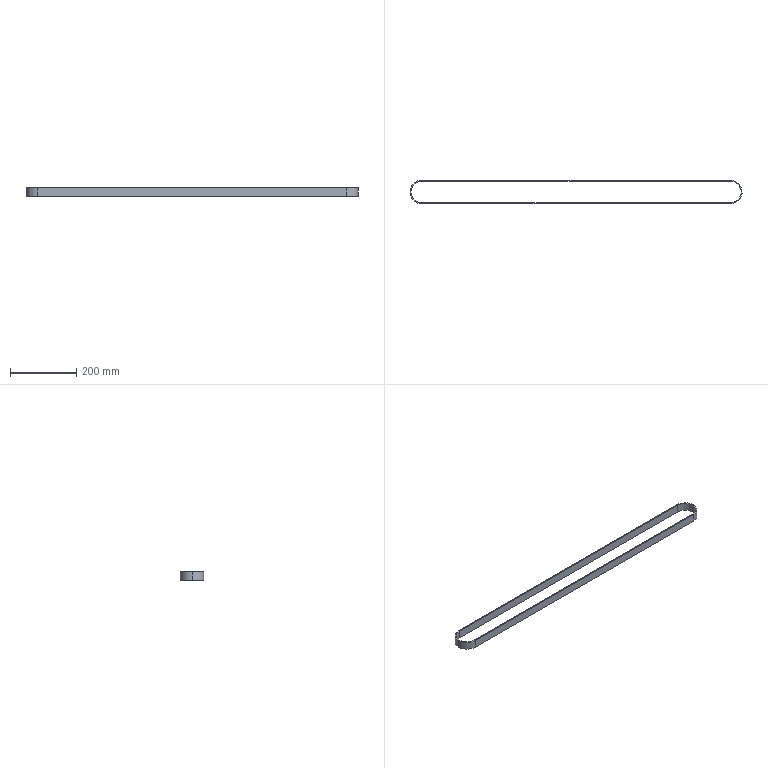Part | STEP file | Timing belt | 1 solid | 12 faces | box 1001 x 71 x 25 mm | volume 155522 mm3 | cylinder 6 | plane 6 | commonest cylinder face diameters 65 x3 71 x3
STEP:
#1=CARTESIAN_POINT('',(-34.001,0.7196,25.));
#2=VERTEX_POINT('',#1);
#3=CARTESIAN_POINT('',(1.594,-34.78,25.));
#4=VERTEX_POINT('',#3);
#5=CARTESIAN_POINT('',(1.499,0.7196,25.));
#6=DIRECTION('',(0.,0.,1.));
#7=DIRECTION('',(-1.,0.,0.));
#8=AXIS2_PLACEMENT_3D('',#5,#6,#7);
#9=CIRCLE('',#8,35.5);
#10=EDGE_CURVE('',#2,#4,#9,.T.);
#11=ORIENTED_EDGE('',*,*,#10,.F.);
#12=CARTESIAN_POINT('',(-34.001,0.7196,0.));
#13=VERTEX_POINT('',#12);
#14=CARTESIAN_POINT('',(-34.001,0.7196,25.));
#15=DIRECTION('',(0.,0.,-1.));
#16=VECTOR('',#15,1000.);
#17=LINE('',#14,#16);
#18=EDGE_CURVE('',#2,#13,#17,.T.);
#19=ORIENTED_EDGE('',*,*,#18,.T.);
#20=CARTESIAN_POINT('',(1.594,-34.78,0.));
#21=VERTEX_POINT('',#20);
#22=CARTESIAN_POINT('',(1.499,0.7196,0.));
#23=DIRECTION('',(0.,0.,1.));
#24=DIRECTION('',(-1.,0.,0.));
#25=AXIS2_PLACEMENT_3D('',#22,#23,#24);
#26=CIRCLE('',#25,35.5);
#27=EDGE_CURVE('',#13,#21,#26,.T.);
#28=ORIENTED_EDGE('',*,*,#27,.T.);
#29=CARTESIAN_POINT('',(1.594,-34.78,25.));
#30=DIRECTION('',(0.,0.,1.));
#31=VECTOR('',#30,1000.);
#32=LINE('',#29,#31);
#33=EDGE_CURVE('',#21,#4,#32,.T.);
#34=ORIENTED_EDGE('',*,*,#33,.T.);
#35=EDGE_LOOP('',(#11,#19,#28,#34));
#36=FACE_OUTER_BOUND('',#35,.T.);
#37=CARTESIAN_POINT('',(1.499,0.7196,25.));
#38=DIRECTION('',(0.,0.,-1.));
#39=DIRECTION('',(-1.,0.,0.));
#40=AXIS2_PLACEMENT_3D('',#37,#38,#39);
#41=CYLINDRICAL_SURFACE('',#40,35.5);
#42=ADVANCED_FACE('',(#36),#41,.T.);
#43=CARTESIAN_POINT('',(-31.001,0.7196,25.));
#44=VERTEX_POINT('',#43);
#45=CARTESIAN_POINT('',(1.411,33.219,25.));
#46=VERTEX_POINT('',#45);
#47=CARTESIAN_POINT('',(1.499,0.7196,25.));
#48=DIRECTION('',(0.,0.,-1.));
#49=DIRECTION('',(-1.,0.,0.));
#50=AXIS2_PLACEMENT_3D('',#47,#48,#49);
#51=CIRCLE('',#50,32.5);
#52=EDGE_CURVE('',#44,#46,#51,.T.);
#53=ORIENTED_EDGE('',*,*,#52,.F.);
#54=CARTESIAN_POINT('',(-31.001,0.7196,0.));
#55=VERTEX_POINT('',#54);
#56=CARTESIAN_POINT('',(-31.001,0.7196,25.));
#57=DIRECTION('',(0.,0.,-1.));
#58=VECTOR('',#57,1000.);
#59=LINE('',#56,#58);
#60=EDGE_CURVE('',#44,#55,#59,.T.);
#61=ORIENTED_EDGE('',*,*,#60,.T.);
#62=CARTESIAN_POINT('',(1.411,33.219,0.));
#63=VERTEX_POINT('',#62);
#64=CARTESIAN_POINT('',(1.499,0.7196,0.));
#65=DIRECTION('',(0.,0.,-1.));
#66=DIRECTION('',(-1.,0.,0.));
#67=AXIS2_PLACEMENT_3D('',#64,#65,#66);
#68=CIRCLE('',#67,32.5);
#69=EDGE_CURVE('',#55,#63,#68,.T.);
#70=ORIENTED_EDGE('',*,*,#69,.T.);
#71=CARTESIAN_POINT('',(1.411,33.219,25.));
#72=DIRECTION('',(0.,0.,-1.));
#73=VECTOR('',#72,1000.);
#74=LINE('',#71,#73);
#75=EDGE_CURVE('',#46,#63,#74,.T.);
#76=ORIENTED_EDGE('',*,*,#75,.F.);
#77=EDGE_LOOP('',(#53,#61,#70,#76));
#78=FACE_OUTER_BOUND('',#77,.T.);
#79=CARTESIAN_POINT('',(1.499,0.7196,25.));
#80=DIRECTION('',(0.,0.,-1.));
#81=DIRECTION('',(-1.,0.,0.));
#82=AXIS2_PLACEMENT_3D('',#79,#80,#81);
#83=CYLINDRICAL_SURFACE('',#82,32.5);
#84=ADVANCED_FACE('',(#78),#83,.F.);
#85=CARTESIAN_POINT('',(931.594,-34.78,25.));
#86=VERTEX_POINT('',#85);
#87=CARTESIAN_POINT('',(931.594,-34.78,0.));
#88=VERTEX_POINT('',#87);
#89=CARTESIAN_POINT('',(931.594,-34.78,25.));
#90=DIRECTION('',(0.,0.,-1.));
#91=VECTOR('',#90,1000.);
#92=LINE('',#89,#91);
#93=EDGE_CURVE('',#86,#88,#92,.T.);
#94=ORIENTED_EDGE('',*,*,#93,.F.);
#95=CARTESIAN_POINT('',(931.594,-34.78,25.));
#96=DIRECTION('',(1.,0.,0.));
#97=VECTOR('',#96,1000.);
#98=LINE('',#95,#97);
#99=EDGE_CURVE('',#4,#86,#98,.T.);
#100=ORIENTED_EDGE('',*,*,#99,.F.);
#101=ORIENTED_EDGE('',*,*,#33,.F.);
#102=CARTESIAN_POINT('',(931.594,-34.78,0.));
#103=DIRECTION('',(-1.,0.,0.));
#104=VECTOR('',#103,1000.);
#105=LINE('',#102,#104);
#106=EDGE_CURVE('',#88,#21,#105,.T.);
#107=ORIENTED_EDGE('',*,*,#106,.F.);
#108=EDGE_LOOP('',(#94,#100,#101,#107));
#109=FACE_OUTER_BOUND('',#108,.T.);
#110=CARTESIAN_POINT('',(931.594,-34.78,25.));
#111=DIRECTION('',(0.,1.,0.));
#112=DIRECTION('',(-1.,0.,0.));
#113=AXIS2_PLACEMENT_3D('',#110,#111,#112);
#114=PLANE('',#113);
#115=ADVANCED_FACE('',(#109),#114,.F.);
#116=CARTESIAN_POINT('',(1.586,-31.78,0.));
#117=VERTEX_POINT('',#116);
#118=CARTESIAN_POINT('',(1.499,0.7196,0.));
#119=DIRECTION('',(0.,0.,-1.));
#120=DIRECTION('',(-1.,0.,0.));
#121=AXIS2_PLACEMENT_3D('',#118,#119,#120);
#122=CIRCLE('',#121,32.5);
#123=EDGE_CURVE('',#117,#55,#122,.T.);
#124=ORIENTED_EDGE('',*,*,#123,.F.);
#125=CARTESIAN_POINT('',(931.586,-31.78,0.));
#126=VERTEX_POINT('',#125);
#127=CARTESIAN_POINT('',(1.499,-31.78,0.));
#128=DIRECTION('',(-1.,0.,0.));
#129=VECTOR('',#128,1000.);
#130=LINE('',#127,#129);
#131=EDGE_CURVE('',#126,#117,#130,.T.);
#132=ORIENTED_EDGE('',*,*,#131,.F.);
#133=CARTESIAN_POINT('',(931.411,33.219,0.));
#134=VERTEX_POINT('',#133);
#135=CARTESIAN_POINT('',(931.499,0.7196,0.));
#136=DIRECTION('',(0.,0.,-1.));
#137=DIRECTION('',(-1.,0.,0.));
#138=AXIS2_PLACEMENT_3D('',#135,#136,#137);
#139=CIRCLE('',#138,32.5);
#140=EDGE_CURVE('',#134,#126,#139,.T.);
#141=ORIENTED_EDGE('',*,*,#140,.F.);
#142=CARTESIAN_POINT('',(1.499,33.219,0.));
#143=DIRECTION('',(1.,0.,0.));
#144=VECTOR('',#143,1000.);
#145=LINE('',#142,#144);
#146=EDGE_CURVE('',#63,#134,#145,.T.);
#147=ORIENTED_EDGE('',*,*,#146,.F.);
#148=ORIENTED_EDGE('',*,*,#69,.F.);
#149=EDGE_LOOP('',(#124,#132,#141,#147,#148));
#150=FACE_BOUND('',#149,.T.);
#151=CARTESIAN_POINT('',(931.403,36.219,0.));
#152=VERTEX_POINT('',#151);
#153=CARTESIAN_POINT('',(1.403,36.219,0.));
#154=VERTEX_POINT('',#153);
#155=CARTESIAN_POINT('',(1.499,36.219,0.));
#156=DIRECTION('',(-1.,0.,0.));
#157=VECTOR('',#156,1000.);
#158=LINE('',#155,#157);
#159=EDGE_CURVE('',#152,#154,#158,.T.);
#160=ORIENTED_EDGE('',*,*,#159,.F.);
#161=CARTESIAN_POINT('',(931.499,0.7196,0.));
#162=DIRECTION('',(0.,0.,1.));
#163=DIRECTION('',(-1.,0.,0.));
#164=AXIS2_PLACEMENT_3D('',#161,#162,#163);
#165=CIRCLE('',#164,35.5);
#166=EDGE_CURVE('',#88,#152,#165,.T.);
#167=ORIENTED_EDGE('',*,*,#166,.F.);
#168=ORIENTED_EDGE('',*,*,#106,.T.);
#169=ORIENTED_EDGE('',*,*,#27,.F.);
#170=CARTESIAN_POINT('',(1.499,0.7196,0.));
#171=DIRECTION('',(0.,0.,1.));
#172=DIRECTION('',(-1.,0.,0.));
#173=AXIS2_PLACEMENT_3D('',#170,#171,#172);
#174=CIRCLE('',#173,35.5);
#175=EDGE_CURVE('',#154,#13,#174,.T.);
#176=ORIENTED_EDGE('',*,*,#175,.F.);
#177=EDGE_LOOP('',(#160,#167,#168,#169,#176));
#178=FACE_OUTER_BOUND('',#177,.T.);
#179=CARTESIAN_POINT('',(1.499,0.7196,0.));
#180=DIRECTION('',(0.,0.,1.));
#181=DIRECTION('',(1.,0.,0.));
#182=AXIS2_PLACEMENT_3D('',#179,#180,#181);
#183=PLANE('',#182);
#184=ADVANCED_FACE('',(#150,#178),#183,.F.);
#185=CARTESIAN_POINT('',(931.403,36.219,25.));
#186=VERTEX_POINT('',#185);
#187=CARTESIAN_POINT('',(931.499,0.7196,25.));
#188=DIRECTION('',(0.,0.,-1.));
#189=DIRECTION('',(-1.,0.,0.));
#190=AXIS2_PLACEMENT_3D('',#187,#188,#189);
#191=CIRCLE('',#190,35.5);
#192=EDGE_CURVE('',#186,#86,#191,.T.);
#193=ORIENTED_EDGE('',*,*,#192,.T.);
#194=ORIENTED_EDGE('',*,*,#93,.T.);
#195=ORIENTED_EDGE('',*,*,#166,.T.);
#196=CARTESIAN_POINT('',(931.403,36.219,25.));
#197=DIRECTION('',(0.,0.,1.));
#198=VECTOR('',#197,1000.);
#199=LINE('',#196,#198);
#200=EDGE_CURVE('',#152,#186,#199,.T.);
#201=ORIENTED_EDGE('',*,*,#200,.T.);
#202=EDGE_LOOP('',(#193,#194,#195,#201));
#203=FACE_OUTER_BOUND('',#202,.T.);
#204=CARTESIAN_POINT('',(931.499,0.7196,25.));
#205=DIRECTION('',(0.,0.,-1.));
#206=DIRECTION('',(-1.,0.,0.));
#207=AXIS2_PLACEMENT_3D('',#204,#205,#206);
#208=CYLINDRICAL_SURFACE('',#207,35.5);
#209=ADVANCED_FACE('',(#203),#208,.T.);
#210=CARTESIAN_POINT('',(931.411,33.219,25.));
#211=VERTEX_POINT('',#210);
#212=CARTESIAN_POINT('',(1.499,33.219,25.));
#213=DIRECTION('',(1.,0.,0.));
#214=VECTOR('',#213,1000.);
#215=LINE('',#212,#214);
#216=EDGE_CURVE('',#46,#211,#215,.T.);
#217=ORIENTED_EDGE('',*,*,#216,.T.);
#218=CARTESIAN_POINT('',(931.586,-31.78,25.));
#219=VERTEX_POINT('',#218);
#220=CARTESIAN_POINT('',(931.499,0.7196,25.));
#221=DIRECTION('',(0.,0.,-1.));
#222=DIRECTION('',(-1.,0.,0.));
#223=AXIS2_PLACEMENT_3D('',#220,#221,#222);
#224=CIRCLE('',#223,32.5);
#225=EDGE_CURVE('',#211,#219,#224,.T.);
#226=ORIENTED_EDGE('',*,*,#225,.T.);
#227=CARTESIAN_POINT('',(1.586,-31.78,25.));
#228=VERTEX_POINT('',#227);
#229=CARTESIAN_POINT('',(1.499,-31.78,25.));
#230=DIRECTION('',(-1.,0.,0.));
#231=VECTOR('',#230,1000.);
#232=LINE('',#229,#231);
#233=EDGE_CURVE('',#219,#228,#232,.T.);
#234=ORIENTED_EDGE('',*,*,#233,.T.);
#235=CARTESIAN_POINT('',(1.499,0.7196,25.));
#236=DIRECTION('',(0.,0.,-1.));
#237=DIRECTION('',(-1.,0.,0.));
#238=AXIS2_PLACEMENT_3D('',#235,#236,#237);
#239=CIRCLE('',#238,32.5);
#240=EDGE_CURVE('',#228,#44,#239,.T.);
#241=ORIENTED_EDGE('',*,*,#240,.T.);
#242=ORIENTED_EDGE('',*,*,#52,.T.);
#243=EDGE_LOOP('',(#217,#226,#234,#241,#242));
#244=FACE_BOUND('',#243,.T.);
#245=ORIENTED_EDGE('',*,*,#192,.F.);
#246=CARTESIAN_POINT('',(1.403,36.219,25.));
#247=VERTEX_POINT('',#246);
#248=CARTESIAN_POINT('',(1.499,36.219,25.));
#249=DIRECTION('',(-1.,0.,0.));
#250=VECTOR('',#249,1000.);
#251=LINE('',#248,#250);
#252=EDGE_CURVE('',#186,#247,#251,.T.);
#253=ORIENTED_EDGE('',*,*,#252,.T.);
#254=CARTESIAN_POINT('',(1.499,0.7196,25.));
#255=DIRECTION('',(0.,0.,1.));
#256=DIRECTION('',(-1.,0.,0.));
#257=AXIS2_PLACEMENT_3D('',#254,#255,#256);
#258=CIRCLE('',#257,35.5);
#259=EDGE_CURVE('',#247,#2,#258,.T.);
#260=ORIENTED_EDGE('',*,*,#259,.T.);
#261=ORIENTED_EDGE('',*,*,#10,.T.);
#262=ORIENTED_EDGE('',*,*,#99,.T.);
#263=EDGE_LOOP('',(#245,#253,#260,#261,#262));
#264=FACE_OUTER_BOUND('',#263,.T.);
#265=CARTESIAN_POINT('',(1.499,0.7196,25.));
#266=DIRECTION('',(0.,0.,1.));
#267=DIRECTION('',(1.,0.,0.));
#268=AXIS2_PLACEMENT_3D('',#265,#266,#267);
#269=PLANE('',#268);
#270=ADVANCED_FACE('',(#244,#264),#269,.T.);
#271=ORIENTED_EDGE('',*,*,#18,.F.);
#272=ORIENTED_EDGE('',*,*,#259,.F.);
#273=CARTESIAN_POINT('',(1.403,36.219,25.));
#274=DIRECTION('',(0.,0.,-1.));
#275=VECTOR('',#274,1000.);
#276=LINE('',#273,#275);
#277=EDGE_CURVE('',#247,#154,#276,.T.);
#278=ORIENTED_EDGE('',*,*,#277,.T.);
#279=ORIENTED_EDGE('',*,*,#175,.T.);
#280=EDGE_LOOP('',(#271,#272,#278,#279));
#281=FACE_OUTER_BOUND('',#280,.T.);
#282=CARTESIAN_POINT('',(1.499,0.7196,25.));
#283=DIRECTION('',(0.,0.,-1.));
#284=DIRECTION('',(-1.,0.,0.));
#285=AXIS2_PLACEMENT_3D('',#282,#283,#284);
#286=CYLINDRICAL_SURFACE('',#285,35.5);
#287=ADVANCED_FACE('',(#281),#286,.T.);
#288=ORIENTED_EDGE('',*,*,#60,.F.);
#289=ORIENTED_EDGE('',*,*,#240,.F.);
#290=CARTESIAN_POINT('',(1.586,-31.78,25.));
#291=DIRECTION('',(0.,0.,1.));
#292=VECTOR('',#291,1000.);
#293=LINE('',#290,#292);
#294=EDGE_CURVE('',#117,#228,#293,.T.);
#295=ORIENTED_EDGE('',*,*,#294,.F.);
#296=ORIENTED_EDGE('',*,*,#123,.T.);
#297=EDGE_LOOP('',(#288,#289,#295,#296));
#298=FACE_OUTER_BOUND('',#297,.T.);
#299=CARTESIAN_POINT('',(1.499,0.7196,25.));
#300=DIRECTION('',(0.,0.,-1.));
#301=DIRECTION('',(-1.,0.,0.));
#302=AXIS2_PLACEMENT_3D('',#299,#300,#301);
#303=CYLINDRICAL_SURFACE('',#302,32.5);
#304=ADVANCED_FACE('',(#298),#303,.F.);
#305=ORIENTED_EDGE('',*,*,#233,.F.);
#306=CARTESIAN_POINT('',(931.586,-31.78,25.));
#307=DIRECTION('',(0.,0.,-1.));
#308=VECTOR('',#307,1000.);
#309=LINE('',#306,#308);
#310=EDGE_CURVE('',#219,#126,#309,.T.);
#311=ORIENTED_EDGE('',*,*,#310,.T.);
#312=ORIENTED_EDGE('',*,*,#131,.T.);
#313=ORIENTED_EDGE('',*,*,#294,.T.);
#314=EDGE_LOOP('',(#305,#311,#312,#313));
#315=FACE_OUTER_BOUND('',#314,.T.);
#316=CARTESIAN_POINT('',(1.586,-31.78,25.));
#317=DIRECTION('',(0.,1.,0.));
#318=DIRECTION('',(-1.,0.,0.));
#319=AXIS2_PLACEMENT_3D('',#316,#317,#318);
#320=PLANE('',#319);
#321=ADVANCED_FACE('',(#315),#320,.T.);
#322=ORIENTED_EDGE('',*,*,#310,.F.);
#323=ORIENTED_EDGE('',*,*,#225,.F.);
#324=CARTESIAN_POINT('',(931.411,33.219,25.));
#325=DIRECTION('',(0.,0.,1.));
#326=VECTOR('',#325,1000.);
#327=LINE('',#324,#326);
#328=EDGE_CURVE('',#134,#211,#327,.T.);
#329=ORIENTED_EDGE('',*,*,#328,.F.);
#330=ORIENTED_EDGE('',*,*,#140,.T.);
#331=EDGE_LOOP('',(#322,#323,#329,#330));
#332=FACE_OUTER_BOUND('',#331,.T.);
#333=CARTESIAN_POINT('',(931.499,0.7196,25.));
#334=DIRECTION('',(0.,0.,-1.));
#335=DIRECTION('',(-1.,0.,0.));
#336=AXIS2_PLACEMENT_3D('',#333,#334,#335);
#337=CYLINDRICAL_SURFACE('',#336,32.5);
#338=ADVANCED_FACE('',(#332),#337,.F.);
#339=ORIENTED_EDGE('',*,*,#216,.F.);
#340=ORIENTED_EDGE('',*,*,#75,.T.);
#341=ORIENTED_EDGE('',*,*,#146,.T.);
#342=ORIENTED_EDGE('',*,*,#328,.T.);
#343=EDGE_LOOP('',(#339,#340,#341,#342));
#344=FACE_OUTER_BOUND('',#343,.T.);
#345=CARTESIAN_POINT('',(1.411,33.219,25.));
#346=DIRECTION('',(0.,-1.,0.));
#347=DIRECTION('',(1.,0.,0.));
#348=AXIS2_PLACEMENT_3D('',#345,#346,#347);
#349=PLANE('',#348);
#350=ADVANCED_FACE('',(#344),#349,.T.);
#351=ORIENTED_EDGE('',*,*,#277,.F.);
#352=ORIENTED_EDGE('',*,*,#252,.F.);
#353=ORIENTED_EDGE('',*,*,#200,.F.);
#354=ORIENTED_EDGE('',*,*,#159,.T.);
#355=EDGE_LOOP('',(#351,#352,#353,#354));
#356=FACE_OUTER_BOUND('',#355,.T.);
#357=CARTESIAN_POINT('',(1.403,36.219,25.));
#358=DIRECTION('',(0.,-1.,0.));
#359=DIRECTION('',(1.,0.,0.));
#360=AXIS2_PLACEMENT_3D('',#357,#358,#359);
#361=PLANE('',#360);
#362=ADVANCED_FACE('',(#356),#361,.F.);
#363=CLOSED_SHELL('',(#42,#84,#115,#184,#209,#270,#287,#304,#321,#338,#350,#362));
#364=MANIFOLD_SOLID_BREP('',#363);
#365=CARTESIAN_POINT('',(0.,0.,0.));
#366=DIRECTION('',(0.,0.,1.));
#367=DIRECTION('',(1.,0.,0.));
#368=AXIS2_PLACEMENT_3D('',#365,#366,#367);
#369=(LENGTH_UNIT()NAMED_UNIT(*)SI_UNIT(.MILLI.,.METRE.));
#370=UNCERTAINTY_MEASURE_WITH_UNIT(LENGTH_MEASURE(0.00001),#369,'','');
#371=(NAMED_UNIT(*)PLANE_ANGLE_UNIT()SI_UNIT($,.RADIAN.));
#372=(NAMED_UNIT(*)SI_UNIT($,.STERADIAN.)SOLID_ANGLE_UNIT());
#373=(GEOMETRIC_REPRESENTATION_CONTEXT(3)GLOBAL_UNCERTAINTY_ASSIGNED_CONTEXT((#370))GLOBAL_UNIT_ASSIGNED_CONTEXT((#369,#371,#372))REPRESENTATION_CONTEXT('',''));
#374=ADVANCED_BREP_SHAPE_REPRESENTATION('',(#364,#368),#373);